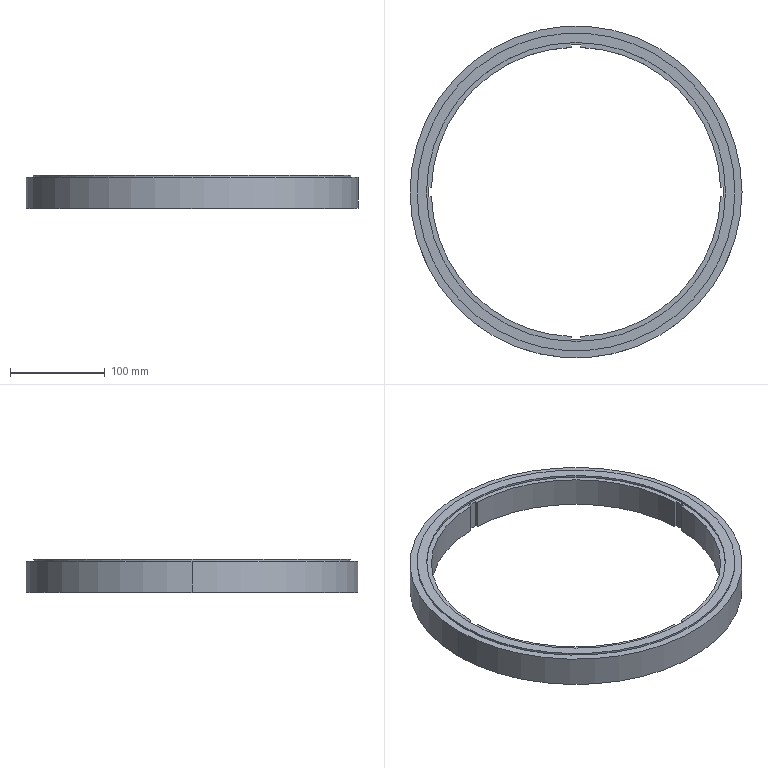Part | SolidWorks | features ICE 6, CirPattern 1, Extrusion 1 | 1 solid | 31 faces | box 350 x 350 x 35 mm | volume 761867 mm3 | plane 17 | cylinder 12 | cone 2 | commonest cylinder face diameters 305 x4 315 x2 330 x2 335 x2 350 x2
STEP:
#1=CARTESIAN_POINT('',(172.,0.,0.));
#2=VERTEX_POINT('',#1);
#3=CARTESIAN_POINT('',(-172.,0.,0.));
#4=VERTEX_POINT('',#3);
#5=CARTESIAN_POINT('',(0.,0.,0.));
#6=DIRECTION('',(0.,0.,-1.));
#7=DIRECTION('',(-1.,0.,0.));
#8=AXIS2_PLACEMENT_3D('',#5,#6,#7);
#9=CIRCLE('',#8,172.);
#10=EDGE_CURVE('',#2,#4,#9,.T.);
#11=ORIENTED_EDGE('',*,*,#10,.F.);
#12=CARTESIAN_POINT('',(175.,0.,0.3684));
#13=VERTEX_POINT('',#12);
#14=CARTESIAN_POINT('',(172.,0.,0.));
#15=DIRECTION('',(0.9925,0.,0.1219));
#16=VECTOR('',#15,1000.);
#17=LINE('',#14,#16);
#18=EDGE_CURVE('',#2,#13,#17,.T.);
#19=ORIENTED_EDGE('',*,*,#18,.T.);
#20=CARTESIAN_POINT('',(-175.,0.,0.3684));
#21=VERTEX_POINT('',#20);
#22=CARTESIAN_POINT('',(0.,0.,0.3684));
#23=DIRECTION('',(0.,0.,-1.));
#24=DIRECTION('',(1.,0.,0.));
#25=AXIS2_PLACEMENT_3D('',#22,#23,#24);
#26=CIRCLE('',#25,175.);
#27=EDGE_CURVE('',#13,#21,#26,.T.);
#28=ORIENTED_EDGE('',*,*,#27,.T.);
#29=CARTESIAN_POINT('',(-172.,0.,0.));
#30=DIRECTION('',(-0.9925,0.,0.1219));
#31=VECTOR('',#30,1000.);
#32=LINE('',#29,#31);
#33=EDGE_CURVE('',#4,#21,#32,.T.);
#34=ORIENTED_EDGE('',*,*,#33,.F.);
#35=EDGE_LOOP('',(#11,#19,#28,#34));
#36=FACE_OUTER_BOUND('',#35,.T.);
#37=CARTESIAN_POINT('',(0.,0.,0.));
#38=DIRECTION('',(0.,0.,1.));
#39=DIRECTION('',(-1.,0.,0.));
#40=AXIS2_PLACEMENT_3D('',#37,#38,#39);
#41=CONICAL_SURFACE('',#40,172.,1.449);
#42=ADVANCED_FACE('',(#36),#41,.T.);
#43=CARTESIAN_POINT('',(165.,0.,1.5));
#44=VERTEX_POINT('',#43);
#45=CARTESIAN_POINT('',(-165.,0.,1.5));
#46=VERTEX_POINT('',#45);
#47=CARTESIAN_POINT('',(0.,0.,1.5));
#48=DIRECTION('',(0.,0.,-1.));
#49=DIRECTION('',(-1.,0.,0.));
#50=AXIS2_PLACEMENT_3D('',#47,#48,#49);
#51=CIRCLE('',#50,165.);
#52=EDGE_CURVE('',#44,#46,#51,.T.);
#53=ORIENTED_EDGE('',*,*,#52,.F.);
#54=CARTESIAN_POINT('',(165.,0.,0.));
#55=VERTEX_POINT('',#54);
#56=CARTESIAN_POINT('',(165.,0.,1.5));
#57=DIRECTION('',(0.,0.,-1.));
#58=VECTOR('',#57,1000.);
#59=LINE('',#56,#58);
#60=EDGE_CURVE('',#44,#55,#59,.T.);
#61=ORIENTED_EDGE('',*,*,#60,.T.);
#62=CARTESIAN_POINT('',(-165.,0.,0.));
#63=VERTEX_POINT('',#62);
#64=CARTESIAN_POINT('',(0.,0.,0.));
#65=DIRECTION('',(0.,0.,-1.));
#66=DIRECTION('',(-1.,0.,0.));
#67=AXIS2_PLACEMENT_3D('',#64,#65,#66);
#68=CIRCLE('',#67,165.);
#69=EDGE_CURVE('',#55,#63,#68,.T.);
#70=ORIENTED_EDGE('',*,*,#69,.T.);
#71=CARTESIAN_POINT('',(-165.,0.,1.5));
#72=DIRECTION('',(0.,0.,-1.));
#73=VECTOR('',#72,1000.);
#74=LINE('',#71,#73);
#75=EDGE_CURVE('',#46,#63,#74,.T.);
#76=ORIENTED_EDGE('',*,*,#75,.F.);
#77=EDGE_LOOP('',(#53,#61,#70,#76));
#78=FACE_OUTER_BOUND('',#77,.T.);
#79=CARTESIAN_POINT('',(0.,0.,1.5));
#80=DIRECTION('',(0.,0.,-1.));
#81=DIRECTION('',(-1.,0.,0.));
#82=AXIS2_PLACEMENT_3D('',#79,#80,#81);
#83=CYLINDRICAL_SURFACE('',#82,165.);
#84=ADVANCED_FACE('',(#78),#83,.F.);
#85=CARTESIAN_POINT('',(-157.5,0.,33.));
#86=VERTEX_POINT('',#85);
#87=CARTESIAN_POINT('',(157.5,0.,33.));
#88=VERTEX_POINT('',#87);
#89=CARTESIAN_POINT('',(0.,0.,33.));
#90=DIRECTION('',(0.,0.,1.));
#91=DIRECTION('',(1.,0.,0.));
#92=AXIS2_PLACEMENT_3D('',#89,#90,#91);
#93=CIRCLE('',#92,157.5);
#94=EDGE_CURVE('',#86,#88,#93,.T.);
#95=ORIENTED_EDGE('',*,*,#94,.F.);
#96=CARTESIAN_POINT('',(-157.5,0.,35.));
#97=VERTEX_POINT('',#96);
#98=CARTESIAN_POINT('',(-157.5,0.,33.));
#99=DIRECTION('',(0.,0.,1.));
#100=VECTOR('',#99,1000.);
#101=LINE('',#98,#100);
#102=EDGE_CURVE('',#86,#97,#101,.T.);
#103=ORIENTED_EDGE('',*,*,#102,.T.);
#104=CARTESIAN_POINT('',(157.5,0.,35.));
#105=VERTEX_POINT('',#104);
#106=CARTESIAN_POINT('',(0.,0.,35.));
#107=DIRECTION('',(0.,0.,1.));
#108=DIRECTION('',(1.,0.,0.));
#109=AXIS2_PLACEMENT_3D('',#106,#107,#108);
#110=CIRCLE('',#109,157.5);
#111=EDGE_CURVE('',#97,#105,#110,.T.);
#112=ORIENTED_EDGE('',*,*,#111,.T.);
#113=CARTESIAN_POINT('',(157.5,0.,33.));
#114=DIRECTION('',(0.,0.,1.));
#115=VECTOR('',#114,1000.);
#116=LINE('',#113,#115);
#117=EDGE_CURVE('',#88,#105,#116,.T.);
#118=ORIENTED_EDGE('',*,*,#117,.F.);
#119=EDGE_LOOP('',(#95,#103,#112,#118));
#120=FACE_OUTER_BOUND('',#119,.T.);
#121=CARTESIAN_POINT('',(0.,0.,33.));
#122=DIRECTION('',(0.,0.,1.));
#123=DIRECTION('',(1.,0.,0.));
#124=AXIS2_PLACEMENT_3D('',#121,#122,#123);
#125=CYLINDRICAL_SURFACE('',#124,157.5);
#126=ADVANCED_FACE('',(#120),#125,.F.);
#127=CARTESIAN_POINT('',(167.5,0.,33.));
#128=VERTEX_POINT('',#127);
#129=CARTESIAN_POINT('',(-167.5,0.,33.));
#130=VERTEX_POINT('',#129);
#131=CARTESIAN_POINT('',(0.,0.,33.));
#132=DIRECTION('',(0.,0.,1.));
#133=DIRECTION('',(1.,0.,0.));
#134=AXIS2_PLACEMENT_3D('',#131,#132,#133);
#135=CIRCLE('',#134,167.5);
#136=EDGE_CURVE('',#128,#130,#135,.T.);
#137=ORIENTED_EDGE('',*,*,#136,.T.);
#138=CARTESIAN_POINT('',(-167.5,0.,35.));
#139=VERTEX_POINT('',#138);
#140=CARTESIAN_POINT('',(-167.5,0.,33.));
#141=DIRECTION('',(0.,0.,1.));
#142=VECTOR('',#141,1000.);
#143=LINE('',#140,#142);
#144=EDGE_CURVE('',#130,#139,#143,.T.);
#145=ORIENTED_EDGE('',*,*,#144,.T.);
#146=CARTESIAN_POINT('',(167.5,0.,35.));
#147=VERTEX_POINT('',#146);
#148=CARTESIAN_POINT('',(0.,0.,35.));
#149=DIRECTION('',(0.,0.,1.));
#150=DIRECTION('',(1.,0.,0.));
#151=AXIS2_PLACEMENT_3D('',#148,#149,#150);
#152=CIRCLE('',#151,167.5);
#153=EDGE_CURVE('',#147,#139,#152,.T.);
#154=ORIENTED_EDGE('',*,*,#153,.F.);
#155=CARTESIAN_POINT('',(167.5,0.,33.));
#156=DIRECTION('',(0.,0.,1.));
#157=VECTOR('',#156,1000.);
#158=LINE('',#155,#157);
#159=EDGE_CURVE('',#128,#147,#158,.T.);
#160=ORIENTED_EDGE('',*,*,#159,.F.);
#161=EDGE_LOOP('',(#137,#145,#154,#160));
#162=FACE_OUTER_BOUND('',#161,.T.);
#163=CARTESIAN_POINT('',(0.,0.,33.));
#164=DIRECTION('',(0.,0.,1.));
#165=DIRECTION('',(1.,0.,0.));
#166=AXIS2_PLACEMENT_3D('',#163,#164,#165);
#167=CYLINDRICAL_SURFACE('',#166,167.5);
#168=ADVANCED_FACE('',(#162),#167,.T.);
#169=CARTESIAN_POINT('',(175.,0.,33.));
#170=VERTEX_POINT('',#169);
#171=CARTESIAN_POINT('',(-175.,0.,33.));
#172=VERTEX_POINT('',#171);
#173=CARTESIAN_POINT('',(0.,0.,33.));
#174=DIRECTION('',(0.,0.,1.));
#175=DIRECTION('',(1.,0.,0.));
#176=AXIS2_PLACEMENT_3D('',#173,#174,#175);
#177=CIRCLE('',#176,175.);
#178=EDGE_CURVE('',#170,#172,#177,.T.);
#179=ORIENTED_EDGE('',*,*,#178,.F.);
#180=CARTESIAN_POINT('',(175.,0.,35.));
#181=DIRECTION('',(0.,0.,-1.));
#182=VECTOR('',#181,1000.);
#183=LINE('',#180,#182);
#184=EDGE_CURVE('',#170,#13,#183,.T.);
#185=ORIENTED_EDGE('',*,*,#184,.T.);
#186=CARTESIAN_POINT('',(0.,0.,0.3684));
#187=DIRECTION('',(0.,0.,-1.));
#188=DIRECTION('',(1.,0.,0.));
#189=AXIS2_PLACEMENT_3D('',#186,#187,#188);
#190=CIRCLE('',#189,175.);
#191=EDGE_CURVE('',#21,#13,#190,.T.);
#192=ORIENTED_EDGE('',*,*,#191,.F.);
#193=CARTESIAN_POINT('',(-175.,0.,35.));
#194=DIRECTION('',(0.,0.,-1.));
#195=VECTOR('',#194,1000.);
#196=LINE('',#193,#195);
#197=EDGE_CURVE('',#172,#21,#196,.T.);
#198=ORIENTED_EDGE('',*,*,#197,.F.);
#199=EDGE_LOOP('',(#179,#185,#192,#198));
#200=FACE_OUTER_BOUND('',#199,.T.);
#201=CARTESIAN_POINT('',(0.,0.,35.));
#202=DIRECTION('',(0.,0.,-1.));
#203=DIRECTION('',(-1.,0.,0.));
#204=AXIS2_PLACEMENT_3D('',#201,#202,#203);
#205=CYLINDRICAL_SURFACE('',#204,175.);
#206=ADVANCED_FACE('',(#200),#205,.T.);
#207=ORIENTED_EDGE('',*,*,#184,.F.);
#208=CARTESIAN_POINT('',(0.,0.,33.));
#209=DIRECTION('',(0.,0.,1.));
#210=DIRECTION('',(1.,0.,0.));
#211=AXIS2_PLACEMENT_3D('',#208,#209,#210);
#212=CIRCLE('',#211,175.);
#213=EDGE_CURVE('',#172,#170,#212,.T.);
#214=ORIENTED_EDGE('',*,*,#213,.F.);
#215=ORIENTED_EDGE('',*,*,#197,.T.);
#216=ORIENTED_EDGE('',*,*,#27,.F.);
#217=EDGE_LOOP('',(#207,#214,#215,#216));
#218=FACE_OUTER_BOUND('',#217,.T.);
#219=CARTESIAN_POINT('',(0.,0.,35.));
#220=DIRECTION('',(0.,0.,-1.));
#221=DIRECTION('',(-1.,0.,0.));
#222=AXIS2_PLACEMENT_3D('',#219,#220,#221);
#223=CYLINDRICAL_SURFACE('',#222,175.);
#224=ADVANCED_FACE('',(#218),#223,.T.);
#225=CARTESIAN_POINT('',(0.,0.,0.));
#226=DIRECTION('',(0.,0.,-1.));
#227=DIRECTION('',(-1.,0.,0.));
#228=AXIS2_PLACEMENT_3D('',#225,#226,#227);
#229=CIRCLE('',#228,165.);
#230=EDGE_CURVE('',#63,#55,#229,.T.);
#231=ORIENTED_EDGE('',*,*,#230,.F.);
#232=ORIENTED_EDGE('',*,*,#69,.F.);
#233=EDGE_LOOP('',(#231,#232));
#234=FACE_BOUND('',#233,.T.);
#235=CARTESIAN_POINT('',(0.,0.,0.));
#236=DIRECTION('',(0.,0.,-1.));
#237=DIRECTION('',(-1.,0.,0.));
#238=AXIS2_PLACEMENT_3D('',#235,#236,#237);
#239=CIRCLE('',#238,172.);
#240=EDGE_CURVE('',#4,#2,#239,.T.);
#241=ORIENTED_EDGE('',*,*,#240,.T.);
#242=ORIENTED_EDGE('',*,*,#10,.T.);
#243=EDGE_LOOP('',(#241,#242));
#244=FACE_OUTER_BOUND('',#243,.T.);
#245=CARTESIAN_POINT('',(0.,0.,0.));
#246=DIRECTION('',(0.,0.,1.));
#247=DIRECTION('',(1.,0.,0.));
#248=AXIS2_PLACEMENT_3D('',#245,#246,#247);
#249=PLANE('',#248);
#250=ADVANCED_FACE('',(#234,#244),#249,.F.);
#251=CARTESIAN_POINT('',(-5.,-152.418,1.5));
#252=VERTEX_POINT('',#251);
#253=CARTESIAN_POINT('',(-152.418,-5.,1.5));
#254=VERTEX_POINT('',#253);
#255=CARTESIAN_POINT('',(0.,0.,1.5));
#256=DIRECTION('',(0.,0.,-1.));
#257=DIRECTION('',(-1.,0.,0.));
#258=AXIS2_PLACEMENT_3D('',#255,#256,#257);
#259=CIRCLE('',#258,152.5);
#260=EDGE_CURVE('',#252,#254,#259,.T.);
#261=ORIENTED_EDGE('',*,*,#260,.T.);
#262=CARTESIAN_POINT('',(-152.418,-5.,33.));
#263=VERTEX_POINT('',#262);
#264=CARTESIAN_POINT('',(-152.418,-5.,35.));
#265=DIRECTION('',(0.,0.,1.));
#266=VECTOR('',#265,1000.);
#267=LINE('',#264,#266);
#268=EDGE_CURVE('',#254,#263,#267,.T.);
#269=ORIENTED_EDGE('',*,*,#268,.T.);
#270=CARTESIAN_POINT('',(-5.,-152.418,33.));
#271=VERTEX_POINT('',#270);
#272=CARTESIAN_POINT('',(0.,0.,33.));
#273=DIRECTION('',(0.,0.,1.));
#274=DIRECTION('',(1.,0.,0.));
#275=AXIS2_PLACEMENT_3D('',#272,#273,#274);
#276=CIRCLE('',#275,152.5);
#277=EDGE_CURVE('',#263,#271,#276,.T.);
#278=ORIENTED_EDGE('',*,*,#277,.T.);
#279=CARTESIAN_POINT('',(-5.,-152.418,35.));
#280=DIRECTION('',(0.,0.,-1.));
#281=VECTOR('',#280,1000.);
#282=LINE('',#279,#281);
#283=EDGE_CURVE('',#271,#252,#282,.T.);
#284=ORIENTED_EDGE('',*,*,#283,.T.);
#285=EDGE_LOOP('',(#261,#269,#278,#284));
#286=FACE_OUTER_BOUND('',#285,.T.);
#287=CARTESIAN_POINT('',(0.,0.,35.));
#288=DIRECTION('',(0.,0.,-1.));
#289=DIRECTION('',(-1.,0.,0.));
#290=AXIS2_PLACEMENT_3D('',#287,#288,#289);
#291=CYLINDRICAL_SURFACE('',#290,152.5);
#292=ADVANCED_FACE('',(#286),#291,.F.);
#293=CARTESIAN_POINT('',(5.,-152.418,33.));
#294=VERTEX_POINT('',#293);
#295=CARTESIAN_POINT('',(152.418,-5.,33.));
#296=VERTEX_POINT('',#295);
#297=CARTESIAN_POINT('',(0.,0.,33.));
#298=DIRECTION('',(0.,0.,1.));
#299=DIRECTION('',(1.,0.,0.));
#300=AXIS2_PLACEMENT_3D('',#297,#298,#299);
#301=CIRCLE('',#300,152.5);
#302=EDGE_CURVE('',#294,#296,#301,.T.);
#303=ORIENTED_EDGE('',*,*,#302,.T.);
#304=CARTESIAN_POINT('',(152.418,-5.,1.5));
#305=VERTEX_POINT('',#304);
#306=CARTESIAN_POINT('',(152.418,-5.,35.));
#307=DIRECTION('',(0.,0.,-1.));
#308=VECTOR('',#307,1000.);
#309=LINE('',#306,#308);
#310=EDGE_CURVE('',#296,#305,#309,.T.);
#311=ORIENTED_EDGE('',*,*,#310,.T.);
#312=CARTESIAN_POINT('',(5.,-152.418,1.5));
#313=VERTEX_POINT('',#312);
#314=CARTESIAN_POINT('',(0.,0.,1.5));
#315=DIRECTION('',(0.,0.,-1.));
#316=DIRECTION('',(-1.,0.,0.));
#317=AXIS2_PLACEMENT_3D('',#314,#315,#316);
#318=CIRCLE('',#317,152.5);
#319=EDGE_CURVE('',#305,#313,#318,.T.);
#320=ORIENTED_EDGE('',*,*,#319,.T.);
#321=CARTESIAN_POINT('',(5.,-152.418,35.));
#322=DIRECTION('',(0.,0.,1.));
#323=VECTOR('',#322,1000.);
#324=LINE('',#321,#323);
#325=EDGE_CURVE('',#313,#294,#324,.T.);
#326=ORIENTED_EDGE('',*,*,#325,.T.);
#327=EDGE_LOOP('',(#303,#311,#320,#326));
#328=FACE_OUTER_BOUND('',#327,.T.);
#329=CARTESIAN_POINT('',(0.,0.,35.));
#330=DIRECTION('',(0.,0.,-1.));
#331=DIRECTION('',(-1.,0.,0.));
#332=AXIS2_PLACEMENT_3D('',#329,#330,#331);
#333=CYLINDRICAL_SURFACE('',#332,152.5);
#334=ADVANCED_FACE('',(#328),#333,.F.);
#335=CARTESIAN_POINT('',(-5.,152.418,33.));
#336=VERTEX_POINT('',#335);
#337=CARTESIAN_POINT('',(-152.418,5.,33.));
#338=VERTEX_POINT('',#337);
#339=CARTESIAN_POINT('',(0.,0.,33.));
#340=DIRECTION('',(0.,0.,1.));
#341=DIRECTION('',(1.,0.,0.));
#342=AXIS2_PLACEMENT_3D('',#339,#340,#341);
#343=CIRCLE('',#342,152.5);
#344=EDGE_CURVE('',#336,#338,#343,.T.);
#345=ORIENTED_EDGE('',*,*,#344,.T.);
#346=CARTESIAN_POINT('',(-152.418,5.,1.5));
#347=VERTEX_POINT('',#346);
#348=CARTESIAN_POINT('',(-152.418,5.,35.));
#349=DIRECTION('',(0.,0.,-1.));
#350=VECTOR('',#349,1000.);
#351=LINE('',#348,#350);
#352=EDGE_CURVE('',#338,#347,#351,.T.);
#353=ORIENTED_EDGE('',*,*,#352,.T.);
#354=CARTESIAN_POINT('',(-5.,152.418,1.5));
#355=VERTEX_POINT('',#354);
#356=CARTESIAN_POINT('',(0.,0.,1.5));
#357=DIRECTION('',(0.,0.,-1.));
#358=DIRECTION('',(-1.,0.,0.));
#359=AXIS2_PLACEMENT_3D('',#356,#357,#358);
#360=CIRCLE('',#359,152.5);
#361=EDGE_CURVE('',#347,#355,#360,.T.);
#362=ORIENTED_EDGE('',*,*,#361,.T.);
#363=CARTESIAN_POINT('',(-5.,152.418,35.));
#364=DIRECTION('',(0.,0.,1.));
#365=VECTOR('',#364,1000.);
#366=LINE('',#363,#365);
#367=EDGE_CURVE('',#355,#336,#366,.T.);
#368=ORIENTED_EDGE('',*,*,#367,.T.);
#369=EDGE_LOOP('',(#345,#353,#362,#368));
#370=FACE_OUTER_BOUND('',#369,.T.);
#371=CARTESIAN_POINT('',(0.,0.,35.));
#372=DIRECTION('',(0.,0.,-1.));
#373=DIRECTION('',(-1.,0.,0.));
#374=AXIS2_PLACEMENT_3D('',#371,#372,#373);
#375=CYLINDRICAL_SURFACE('',#374,152.5);
#376=ADVANCED_FACE('',(#370),#375,.F.);
#377=ORIENTED_EDGE('',*,*,#136,.F.);
#378=CARTESIAN_POINT('',(0.,0.,33.));
#379=DIRECTION('',(0.,0.,1.));
#380=DIRECTION('',(1.,0.,0.));
#381=AXIS2_PLACEMENT_3D('',#378,#379,#380);
#382=CIRCLE('',#381,167.5);
#383=EDGE_CURVE('',#130,#128,#382,.T.);
#384=ORIENTED_EDGE('',*,*,#383,.F.);
#385=EDGE_LOOP('',(#377,#384));
#386=FACE_BOUND('',#385,.T.);
#387=ORIENTED_EDGE('',*,*,#213,.T.);
#388=ORIENTED_EDGE('',*,*,#178,.T.);
#389=EDGE_LOOP('',(#387,#388));
#390=FACE_OUTER_BOUND('',#389,.T.);
#391=CARTESIAN_POINT('',(0.,0.,33.));
#392=DIRECTION('',(0.,0.,1.));
#393=DIRECTION('',(1.,0.,0.));
#394=AXIS2_PLACEMENT_3D('',#391,#392,#393);
#395=PLANE('',#394);
#396=ADVANCED_FACE('',(#386,#390),#395,.T.);
#397=ORIENTED_EDGE('',*,*,#144,.F.);
#398=ORIENTED_EDGE('',*,*,#383,.T.);
#399=ORIENTED_EDGE('',*,*,#159,.T.);
#400=CARTESIAN_POINT('',(0.,0.,35.));
#401=DIRECTION('',(0.,0.,1.));
#402=DIRECTION('',(1.,0.,0.));
#403=AXIS2_PLACEMENT_3D('',#400,#401,#402);
#404=CIRCLE('',#403,167.5);
#405=EDGE_CURVE('',#139,#147,#404,.T.);
#406=ORIENTED_EDGE('',*,*,#405,.F.);
#407=EDGE_LOOP('',(#397,#398,#399,#406));
#408=FACE_OUTER_BOUND('',#407,.T.);
#409=CARTESIAN_POINT('',(0.,0.,33.));
#410=DIRECTION('',(0.,0.,1.));
#411=DIRECTION('',(1.,0.,0.));
#412=AXIS2_PLACEMENT_3D('',#409,#410,#411);
#413=CYLINDRICAL_SURFACE('',#412,167.5);
#414=ADVANCED_FACE('',(#408),#413,.T.);
#415=CARTESIAN_POINT('',(0.,0.,35.));
#416=DIRECTION('',(0.,0.,1.));
#417=DIRECTION('',(1.,0.,0.));
#418=AXIS2_PLACEMENT_3D('',#415,#416,#417);
#419=CIRCLE('',#418,157.5);
#420=EDGE_CURVE('',#105,#97,#419,.T.);
#421=ORIENTED_EDGE('',*,*,#420,.F.);
#422=ORIENTED_EDGE('',*,*,#111,.F.);
#423=EDGE_LOOP('',(#421,#422));
#424=FACE_BOUND('',#423,.T.);
#425=ORIENTED_EDGE('',*,*,#153,.T.);
#426=ORIENTED_EDGE('',*,*,#405,.T.);
#427=EDGE_LOOP('',(#425,#426));
#428=FACE_OUTER_BOUND('',#427,.T.);
#429=CARTESIAN_POINT('',(0.,0.,35.));
#430=DIRECTION('',(0.,0.,1.));
#431=DIRECTION('',(1.,0.,0.));
#432=AXIS2_PLACEMENT_3D('',#429,#430,#431);
#433=PLANE('',#432);
#434=ADVANCED_FACE('',(#424,#428),#433,.T.);
#435=ORIENTED_EDGE('',*,*,#102,.F.);
#436=CARTESIAN_POINT('',(0.,0.,33.));
#437=DIRECTION('',(0.,0.,1.));
#438=DIRECTION('',(1.,0.,0.));
#439=AXIS2_PLACEMENT_3D('',#436,#437,#438);
#440=CIRCLE('',#439,157.5);
#441=EDGE_CURVE('',#88,#86,#440,.T.);
#442=ORIENTED_EDGE('',*,*,#441,.F.);
#443=ORIENTED_EDGE('',*,*,#117,.T.);
#444=ORIENTED_EDGE('',*,*,#420,.T.);
#445=EDGE_LOOP('',(#435,#442,#443,#444));
#446=FACE_OUTER_BOUND('',#445,.T.);
#447=CARTESIAN_POINT('',(0.,0.,33.));
#448=DIRECTION('',(0.,0.,1.));
#449=DIRECTION('',(1.,0.,0.));
#450=AXIS2_PLACEMENT_3D('',#447,#448,#449);
#451=CYLINDRICAL_SURFACE('',#450,157.5);
#452=ADVANCED_FACE('',(#446),#451,.F.);
#453=CARTESIAN_POINT('',(155.,-5.,33.));
#454=VERTEX_POINT('',#453);
#455=CARTESIAN_POINT('',(0.,-5.,33.));
#456=DIRECTION('',(1.,0.,0.));
#457=VECTOR('',#456,1000.);
#458=LINE('',#455,#457);
#459=EDGE_CURVE('',#296,#454,#458,.T.);
#460=ORIENTED_EDGE('',*,*,#459,.F.);
#461=ORIENTED_EDGE('',*,*,#302,.F.);
#462=CARTESIAN_POINT('',(5.,-155.,33.));
#463=VERTEX_POINT('',#462);
#464=CARTESIAN_POINT('',(5.,0.,33.));
#465=DIRECTION('',(0.,1.,0.));
#466=VECTOR('',#465,1000.);
#467=LINE('',#464,#466);
#468=EDGE_CURVE('',#463,#294,#467,.T.);
#469=ORIENTED_EDGE('',*,*,#468,.F.);
#470=CARTESIAN_POINT('',(-5.,-155.,33.));
#471=VERTEX_POINT('',#470);
#472=CARTESIAN_POINT('',(0.,-155.,33.));
#473=DIRECTION('',(1.,0.,0.));
#474=VECTOR('',#473,1000.);
#475=LINE('',#472,#474);
#476=EDGE_CURVE('',#471,#463,#475,.T.);
#477=ORIENTED_EDGE('',*,*,#476,.F.);
#478=CARTESIAN_POINT('',(-5.,0.,33.));
#479=DIRECTION('',(0.,-1.,0.));
#480=VECTOR('',#479,1000.);
#481=LINE('',#478,#480);
#482=EDGE_CURVE('',#271,#471,#481,.T.);
#483=ORIENTED_EDGE('',*,*,#482,.F.);
#484=ORIENTED_EDGE('',*,*,#277,.F.);
#485=CARTESIAN_POINT('',(-155.,-5.,33.));
#486=VERTEX_POINT('',#485);
#487=CARTESIAN_POINT('',(0.,-5.,33.));
#488=DIRECTION('',(1.,0.,0.));
#489=VECTOR('',#488,1000.);
#490=LINE('',#487,#489);
#491=EDGE_CURVE('',#486,#263,#490,.T.);
#492=ORIENTED_EDGE('',*,*,#491,.F.);
#493=CARTESIAN_POINT('',(-155.,5.,33.));
#494=VERTEX_POINT('',#493);
#495=CARTESIAN_POINT('',(-155.,0.,33.));
#496=DIRECTION('',(0.,-1.,0.));
#497=VECTOR('',#496,1000.);
#498=LINE('',#495,#497);
#499=EDGE_CURVE('',#494,#486,#498,.T.);
#500=ORIENTED_EDGE('',*,*,#499,.F.);
#501=CARTESIAN_POINT('',(0.,5.,33.));
#502=DIRECTION('',(-1.,0.,0.));
#503=VECTOR('',#502,1000.);
#504=LINE('',#501,#503);
#505=EDGE_CURVE('',#338,#494,#504,.T.);
#506=ORIENTED_EDGE('',*,*,#505,.F.);
#507=ORIENTED_EDGE('',*,*,#344,.F.);
#508=CARTESIAN_POINT('',(-5.,155.,33.));
#509=VERTEX_POINT('',#508);
#510=CARTESIAN_POINT('',(-5.,0.,33.));
#511=DIRECTION('',(0.,-1.,0.));
#512=VECTOR('',#511,1000.);
#513=LINE('',#510,#512);
#514=EDGE_CURVE('',#509,#336,#513,.T.);
#515=ORIENTED_EDGE('',*,*,#514,.F.);
#516=CARTESIAN_POINT('',(5.,155.,33.));
#517=VERTEX_POINT('',#516);
#518=CARTESIAN_POINT('',(0.,155.,33.));
#519=DIRECTION('',(-1.,0.,0.));
#520=VECTOR('',#519,1000.);
#521=LINE('',#518,#520);
#522=EDGE_CURVE('',#517,#509,#521,.T.);
#523=ORIENTED_EDGE('',*,*,#522,.F.);
#524=CARTESIAN_POINT('',(5.,152.418,33.));
#525=VERTEX_POINT('',#524);
#526=CARTESIAN_POINT('',(5.,0.,33.));
#527=DIRECTION('',(0.,1.,0.));
#528=VECTOR('',#527,1000.);
#529=LINE('',#526,#528);
#530=EDGE_CURVE('',#525,#517,#529,.T.);
#531=ORIENTED_EDGE('',*,*,#530,.F.);
#532=CARTESIAN_POINT('',(152.418,5.,33.));
#533=VERTEX_POINT('',#532);
#534=CARTESIAN_POINT('',(0.,0.,33.));
#535=DIRECTION('',(0.,0.,1.));
#536=DIRECTION('',(1.,0.,0.));
#537=AXIS2_PLACEMENT_3D('',#534,#535,#536);
#538=CIRCLE('',#537,152.5);
#539=EDGE_CURVE('',#533,#525,#538,.T.);
#540=ORIENTED_EDGE('',*,*,#539,.F.);
#541=CARTESIAN_POINT('',(155.,5.,33.));
#542=VERTEX_POINT('',#541);
#543=CARTESIAN_POINT('',(0.,5.,33.));
#544=DIRECTION('',(-1.,0.,0.));
#545=VECTOR('',#544,1000.);
#546=LINE('',#543,#545);
#547=EDGE_CURVE('',#542,#533,#546,.T.);
#548=ORIENTED_EDGE('',*,*,#547,.F.);
#549=CARTESIAN_POINT('',(155.,0.,33.));
#550=DIRECTION('',(0.,1.,0.));
#551=VECTOR('',#550,1000.);
#552=LINE('',#549,#551);
#553=EDGE_CURVE('',#454,#542,#552,.T.);
#554=ORIENTED_EDGE('',*,*,#553,.F.);
#555=EDGE_LOOP('',(#460,#461,#469,#477,#483,#484,#492,#500,#506,#507,#515,#523,#531,#540,#548,#554));
#556=FACE_BOUND('',#555,.T.);
#557=ORIENTED_EDGE('',*,*,#441,.T.);
#558=ORIENTED_EDGE('',*,*,#94,.T.);
#559=EDGE_LOOP('',(#557,#558));
#560=FACE_OUTER_BOUND('',#559,.T.);
#561=CARTESIAN_POINT('',(0.,0.,33.));
#562=DIRECTION('',(0.,0.,1.));
#563=DIRECTION('',(1.,0.,0.));
#564=AXIS2_PLACEMENT_3D('',#561,#562,#563);
#565=PLANE('',#564);
#566=ADVANCED_FACE('',(#556,#560),#565,.T.);
#567=ORIENTED_EDGE('',*,*,#60,.F.);
#568=CARTESIAN_POINT('',(0.,0.,1.5));
#569=DIRECTION('',(0.,0.,-1.));
#570=DIRECTION('',(-1.,0.,0.));
#571=AXIS2_PLACEMENT_3D('',#568,#569,#570);
#572=CIRCLE('',#571,165.);
#573=EDGE_CURVE('',#46,#44,#572,.T.);
#574=ORIENTED_EDGE('',*,*,#573,.F.);
#575=ORIENTED_EDGE('',*,*,#75,.T.);
#576=ORIENTED_EDGE('',*,*,#230,.T.);
#577=EDGE_LOOP('',(#567,#574,#575,#576));
#578=FACE_OUTER_BOUND('',#577,.T.);
#579=CARTESIAN_POINT('',(0.,0.,1.5));
#580=DIRECTION('',(0.,0.,-1.));
#581=DIRECTION('',(-1.,0.,0.));
#582=AXIS2_PLACEMENT_3D('',#579,#580,#581);
#583=CYLINDRICAL_SURFACE('',#582,165.);
#584=ADVANCED_FACE('',(#578),#583,.F.);
#585=CARTESIAN_POINT('',(155.,-5.,1.5));
#586=VERTEX_POINT('',#585);
#587=CARTESIAN_POINT('',(155.,-5.,1.5));
#588=DIRECTION('',(-1.,0.,0.));
#589=VECTOR('',#588,1000.);
#590=LINE('',#587,#589);
#591=EDGE_CURVE('',#586,#305,#590,.T.);
#592=ORIENTED_EDGE('',*,*,#591,.F.);
#593=CARTESIAN_POINT('',(155.,5.,1.5));
#594=VERTEX_POINT('',#593);
#595=CARTESIAN_POINT('',(155.,5.,1.5));
#596=DIRECTION('',(0.,-1.,0.));
#597=VECTOR('',#596,1000.);
#598=LINE('',#595,#597);
#599=EDGE_CURVE('',#594,#586,#598,.T.);
#600=ORIENTED_EDGE('',*,*,#599,.F.);
#601=CARTESIAN_POINT('',(152.418,5.,1.5));
#602=VERTEX_POINT('',#601);
#603=CARTESIAN_POINT('',(155.,5.,1.5));
#604=DIRECTION('',(1.,0.,0.));
#605=VECTOR('',#604,1000.);
#606=LINE('',#603,#605);
#607=EDGE_CURVE('',#602,#594,#606,.T.);
#608=ORIENTED_EDGE('',*,*,#607,.F.);
#609=CARTESIAN_POINT('',(5.,152.418,1.5));
#610=VERTEX_POINT('',#609);
#611=CARTESIAN_POINT('',(0.,0.,1.5));
#612=DIRECTION('',(0.,0.,-1.));
#613=DIRECTION('',(-1.,0.,0.));
#614=AXIS2_PLACEMENT_3D('',#611,#612,#613);
#615=CIRCLE('',#614,152.5);
#616=EDGE_CURVE('',#610,#602,#615,.T.);
#617=ORIENTED_EDGE('',*,*,#616,.F.);
#618=CARTESIAN_POINT('',(5.,155.,1.5));
#619=VERTEX_POINT('',#618);
#620=CARTESIAN_POINT('',(5.,-155.,1.5));
#621=DIRECTION('',(0.,-1.,0.));
#622=VECTOR('',#621,1000.);
#623=LINE('',#620,#622);
#624=EDGE_CURVE('',#619,#610,#623,.T.);
#625=ORIENTED_EDGE('',*,*,#624,.F.);
#626=CARTESIAN_POINT('',(-5.,155.,1.5));
#627=VERTEX_POINT('',#626);
#628=CARTESIAN_POINT('',(5.,155.,1.5));
#629=DIRECTION('',(1.,0.,0.));
#630=VECTOR('',#629,1000.);
#631=LINE('',#628,#630);
#632=EDGE_CURVE('',#627,#619,#631,.T.);
#633=ORIENTED_EDGE('',*,*,#632,.F.);
#634=CARTESIAN_POINT('',(-5.,-155.,1.5));
#635=DIRECTION('',(0.,1.,0.));
#636=VECTOR('',#635,1000.);
#637=LINE('',#634,#636);
#638=EDGE_CURVE('',#355,#627,#637,.T.);
#639=ORIENTED_EDGE('',*,*,#638,.F.);
#640=ORIENTED_EDGE('',*,*,#361,.F.);
#641=CARTESIAN_POINT('',(-155.,5.,1.5));
#642=VERTEX_POINT('',#641);
#643=CARTESIAN_POINT('',(155.,5.,1.5));
#644=DIRECTION('',(1.,0.,0.));
#645=VECTOR('',#644,1000.);
#646=LINE('',#643,#645);
#647=EDGE_CURVE('',#642,#347,#646,.T.);
#648=ORIENTED_EDGE('',*,*,#647,.F.);
#649=CARTESIAN_POINT('',(-155.,-5.,1.5));
#650=VERTEX_POINT('',#649);
#651=CARTESIAN_POINT('',(-155.,5.,1.5));
#652=DIRECTION('',(0.,1.,0.));
#653=VECTOR('',#652,1000.);
#654=LINE('',#651,#653);
#655=EDGE_CURVE('',#650,#642,#654,.T.);
#656=ORIENTED_EDGE('',*,*,#655,.F.);
#657=CARTESIAN_POINT('',(155.,-5.,1.5));
#658=DIRECTION('',(-1.,0.,0.));
#659=VECTOR('',#658,1000.);
#660=LINE('',#657,#659);
#661=EDGE_CURVE('',#254,#650,#660,.T.);
#662=ORIENTED_EDGE('',*,*,#661,.F.);
#663=ORIENTED_EDGE('',*,*,#260,.F.);
#664=CARTESIAN_POINT('',(-5.,-155.,1.5));
#665=VERTEX_POINT('',#664);
#666=CARTESIAN_POINT('',(-5.,-155.,1.5));
#667=DIRECTION('',(0.,1.,0.));
#668=VECTOR('',#667,1000.);
#669=LINE('',#666,#668);
#670=EDGE_CURVE('',#665,#252,#669,.T.);
#671=ORIENTED_EDGE('',*,*,#670,.F.);
#672=CARTESIAN_POINT('',(5.,-155.,1.5));
#673=VERTEX_POINT('',#672);
#674=CARTESIAN_POINT('',(5.,-155.,1.5));
#675=DIRECTION('',(-1.,0.,0.));
#676=VECTOR('',#675,1000.);
#677=LINE('',#674,#676);
#678=EDGE_CURVE('',#673,#665,#677,.T.);
#679=ORIENTED_EDGE('',*,*,#678,.F.);
#680=CARTESIAN_POINT('',(5.,-155.,1.5));
#681=DIRECTION('',(0.,-1.,0.));
#682=VECTOR('',#681,1000.);
#683=LINE('',#680,#682);
#684=EDGE_CURVE('',#313,#673,#683,.T.);
#685=ORIENTED_EDGE('',*,*,#684,.F.);
#686=ORIENTED_EDGE('',*,*,#319,.F.);
#687=EDGE_LOOP('',(#592,#600,#608,#617,#625,#633,#639,#640,#648,#656,#662,#663,#671,#679,#685,#686));
#688=FACE_BOUND('',#687,.T.);
#689=ORIENTED_EDGE('',*,*,#573,.T.);
#690=ORIENTED_EDGE('',*,*,#52,.T.);
#691=EDGE_LOOP('',(#689,#690));
#692=FACE_OUTER_BOUND('',#691,.T.);
#693=CARTESIAN_POINT('',(0.,0.,1.5));
#694=DIRECTION('',(0.,0.,-1.));
#695=DIRECTION('',(-1.,0.,0.));
#696=AXIS2_PLACEMENT_3D('',#693,#694,#695);
#697=PLANE('',#696);
#698=ADVANCED_FACE('',(#688,#692),#697,.T.);
#699=ORIENTED_EDGE('',*,*,#616,.T.);
#700=CARTESIAN_POINT('',(152.418,5.,35.));
#701=DIRECTION('',(0.,0.,1.));
#702=VECTOR('',#701,1000.);
#703=LINE('',#700,#702);
#704=EDGE_CURVE('',#602,#533,#703,.T.);
#705=ORIENTED_EDGE('',*,*,#704,.T.);
#706=ORIENTED_EDGE('',*,*,#539,.T.);
#707=CARTESIAN_POINT('',(5.,152.418,35.));
#708=DIRECTION('',(0.,0.,-1.));
#709=VECTOR('',#708,1000.);
#710=LINE('',#707,#709);
#711=EDGE_CURVE('',#525,#610,#710,.T.);
#712=ORIENTED_EDGE('',*,*,#711,.T.);
#713=EDGE_LOOP('',(#699,#705,#706,#712));
#714=FACE_OUTER_BOUND('',#713,.T.);
#715=CARTESIAN_POINT('',(0.,0.,35.));
#716=DIRECTION('',(0.,0.,-1.));
#717=DIRECTION('',(-1.,0.,0.));
#718=AXIS2_PLACEMENT_3D('',#715,#716,#717);
#719=CYLINDRICAL_SURFACE('',#718,152.5);
#720=ADVANCED_FACE('',(#714),#719,.F.);
#721=ORIENTED_EDGE('',*,*,#514,.T.);
#722=ORIENTED_EDGE('',*,*,#367,.F.);
#723=ORIENTED_EDGE('',*,*,#638,.T.);
#724=CARTESIAN_POINT('',(-5.,155.,101.));
#725=DIRECTION('',(0.,0.,-1.));
#726=VECTOR('',#725,1000.);
#727=LINE('',#724,#726);
#728=EDGE_CURVE('',#509,#627,#727,.T.);
#729=ORIENTED_EDGE('',*,*,#728,.F.);
#730=EDGE_LOOP('',(#721,#722,#723,#729));
#731=FACE_OUTER_BOUND('',#730,.T.);
#732=CARTESIAN_POINT('',(-5.,-155.,101.));
#733=DIRECTION('',(-1.,0.,0.));
#734=DIRECTION('',(0.,-1.,0.));
#735=AXIS2_PLACEMENT_3D('',#732,#733,#734);
#736=PLANE('',#735);
#737=ADVANCED_FACE('',(#731),#736,.F.);
#738=ORIENTED_EDGE('',*,*,#530,.T.);
#739=CARTESIAN_POINT('',(5.,155.,101.));
#740=DIRECTION('',(0.,0.,-1.));
#741=VECTOR('',#740,1000.);
#742=LINE('',#739,#741);
#743=EDGE_CURVE('',#517,#619,#742,.T.);
#744=ORIENTED_EDGE('',*,*,#743,.T.);
#745=ORIENTED_EDGE('',*,*,#624,.T.);
#746=ORIENTED_EDGE('',*,*,#711,.F.);
#747=EDGE_LOOP('',(#738,#744,#745,#746));
#748=FACE_OUTER_BOUND('',#747,.T.);
#749=CARTESIAN_POINT('',(5.,-155.,101.));
#750=DIRECTION('',(1.,0.,0.));
#751=DIRECTION('',(0.,0.,-1.));
#752=AXIS2_PLACEMENT_3D('',#749,#750,#751);
#753=PLANE('',#752);
#754=ADVANCED_FACE('',(#748),#753,.F.);
#755=ORIENTED_EDGE('',*,*,#522,.T.);
#756=ORIENTED_EDGE('',*,*,#728,.T.);
#757=ORIENTED_EDGE('',*,*,#632,.T.);
#758=ORIENTED_EDGE('',*,*,#743,.F.);
#759=EDGE_LOOP('',(#755,#756,#757,#758));
#760=FACE_OUTER_BOUND('',#759,.T.);
#761=CARTESIAN_POINT('',(5.,155.,101.));
#762=DIRECTION('',(0.,1.,0.));
#763=DIRECTION('',(-1.,0.,0.));
#764=AXIS2_PLACEMENT_3D('',#761,#762,#763);
#765=PLANE('',#764);
#766=ADVANCED_FACE('',(#760),#765,.F.);
#767=ORIENTED_EDGE('',*,*,#468,.T.);
#768=ORIENTED_EDGE('',*,*,#325,.F.);
#769=ORIENTED_EDGE('',*,*,#684,.T.);
#770=CARTESIAN_POINT('',(5.,-155.,101.));
#771=DIRECTION('',(0.,0.,-1.));
#772=VECTOR('',#771,1000.);
#773=LINE('',#770,#772);
#774=EDGE_CURVE('',#463,#673,#773,.T.);
#775=ORIENTED_EDGE('',*,*,#774,.F.);
#776=EDGE_LOOP('',(#767,#768,#769,#775));
#777=FACE_OUTER_BOUND('',#776,.T.);
#778=CARTESIAN_POINT('',(5.,-155.,101.));
#779=DIRECTION('',(1.,0.,0.));
#780=DIRECTION('',(0.,0.,-1.));
#781=AXIS2_PLACEMENT_3D('',#778,#779,#780);
#782=PLANE('',#781);
#783=ADVANCED_FACE('',(#777),#782,.F.);
#784=ORIENTED_EDGE('',*,*,#482,.T.);
#785=CARTESIAN_POINT('',(-5.,-155.,101.));
#786=DIRECTION('',(0.,0.,-1.));
#787=VECTOR('',#786,1000.);
#788=LINE('',#785,#787);
#789=EDGE_CURVE('',#471,#665,#788,.T.);
#790=ORIENTED_EDGE('',*,*,#789,.T.);
#791=ORIENTED_EDGE('',*,*,#670,.T.);
#792=ORIENTED_EDGE('',*,*,#283,.F.);
#793=EDGE_LOOP('',(#784,#790,#791,#792));
#794=FACE_OUTER_BOUND('',#793,.T.);
#795=CARTESIAN_POINT('',(-5.,-155.,101.));
#796=DIRECTION('',(-1.,0.,0.));
#797=DIRECTION('',(0.,-1.,0.));
#798=AXIS2_PLACEMENT_3D('',#795,#796,#797);
#799=PLANE('',#798);
#800=ADVANCED_FACE('',(#794),#799,.F.);
#801=ORIENTED_EDGE('',*,*,#476,.T.);
#802=ORIENTED_EDGE('',*,*,#774,.T.);
#803=ORIENTED_EDGE('',*,*,#678,.T.);
#804=ORIENTED_EDGE('',*,*,#789,.F.);
#805=EDGE_LOOP('',(#801,#802,#803,#804));
#806=FACE_OUTER_BOUND('',#805,.T.);
#807=CARTESIAN_POINT('',(5.,-155.,101.));
#808=DIRECTION('',(0.,-1.,0.));
#809=DIRECTION('',(0.,0.,-1.));
#810=AXIS2_PLACEMENT_3D('',#807,#808,#809);
#811=PLANE('',#810);
#812=ADVANCED_FACE('',(#806),#811,.F.);
#813=ORIENTED_EDGE('',*,*,#547,.T.);
#814=ORIENTED_EDGE('',*,*,#704,.F.);
#815=ORIENTED_EDGE('',*,*,#607,.T.);
#816=CARTESIAN_POINT('',(155.,5.,101.));
#817=DIRECTION('',(0.,0.,-1.));
#818=VECTOR('',#817,1000.);
#819=LINE('',#816,#818);
#820=EDGE_CURVE('',#542,#594,#819,.T.);
#821=ORIENTED_EDGE('',*,*,#820,.F.);
#822=EDGE_LOOP('',(#813,#814,#815,#821));
#823=FACE_OUTER_BOUND('',#822,.T.);
#824=CARTESIAN_POINT('',(155.,5.,101.));
#825=DIRECTION('',(0.,1.,0.));
#826=DIRECTION('',(-1.,0.,0.));
#827=AXIS2_PLACEMENT_3D('',#824,#825,#826);
#828=PLANE('',#827);
#829=ADVANCED_FACE('',(#823),#828,.F.);
#830=ORIENTED_EDGE('',*,*,#459,.T.);
#831=CARTESIAN_POINT('',(155.,-5.,101.));
#832=DIRECTION('',(0.,0.,-1.));
#833=VECTOR('',#832,1000.);
#834=LINE('',#831,#833);
#835=EDGE_CURVE('',#454,#586,#834,.T.);
#836=ORIENTED_EDGE('',*,*,#835,.T.);
#837=ORIENTED_EDGE('',*,*,#591,.T.);
#838=ORIENTED_EDGE('',*,*,#310,.F.);
#839=EDGE_LOOP('',(#830,#836,#837,#838));
#840=FACE_OUTER_BOUND('',#839,.T.);
#841=CARTESIAN_POINT('',(155.,-5.,101.));
#842=DIRECTION('',(0.,-1.,0.));
#843=DIRECTION('',(1.,0.,0.));
#844=AXIS2_PLACEMENT_3D('',#841,#842,#843);
#845=PLANE('',#844);
#846=ADVANCED_FACE('',(#840),#845,.F.);
#847=ORIENTED_EDGE('',*,*,#553,.T.);
#848=ORIENTED_EDGE('',*,*,#820,.T.);
#849=ORIENTED_EDGE('',*,*,#599,.T.);
#850=ORIENTED_EDGE('',*,*,#835,.F.);
#851=EDGE_LOOP('',(#847,#848,#849,#850));
#852=FACE_OUTER_BOUND('',#851,.T.);
#853=CARTESIAN_POINT('',(155.,5.,101.));
#854=DIRECTION('',(1.,0.,0.));
#855=DIRECTION('',(0.,1.,0.));
#856=AXIS2_PLACEMENT_3D('',#853,#854,#855);
#857=PLANE('',#856);
#858=ADVANCED_FACE('',(#852),#857,.F.);
#859=ORIENTED_EDGE('',*,*,#661,.T.);
#860=CARTESIAN_POINT('',(-155.,-5.,101.));
#861=DIRECTION('',(0.,0.,-1.));
#862=VECTOR('',#861,1000.);
#863=LINE('',#860,#862);
#864=EDGE_CURVE('',#486,#650,#863,.T.);
#865=ORIENTED_EDGE('',*,*,#864,.F.);
#866=ORIENTED_EDGE('',*,*,#491,.T.);
#867=ORIENTED_EDGE('',*,*,#268,.F.);
#868=EDGE_LOOP('',(#859,#865,#866,#867));
#869=FACE_OUTER_BOUND('',#868,.T.);
#870=CARTESIAN_POINT('',(155.,-5.,101.));
#871=DIRECTION('',(0.,-1.,0.));
#872=DIRECTION('',(1.,0.,0.));
#873=AXIS2_PLACEMENT_3D('',#870,#871,#872);
#874=PLANE('',#873);
#875=ADVANCED_FACE('',(#869),#874,.F.);
#876=ORIENTED_EDGE('',*,*,#505,.T.);
#877=CARTESIAN_POINT('',(-155.,5.,101.));
#878=DIRECTION('',(0.,0.,-1.));
#879=VECTOR('',#878,1000.);
#880=LINE('',#877,#879);
#881=EDGE_CURVE('',#494,#642,#880,.T.);
#882=ORIENTED_EDGE('',*,*,#881,.T.);
#883=ORIENTED_EDGE('',*,*,#647,.T.);
#884=ORIENTED_EDGE('',*,*,#352,.F.);
#885=EDGE_LOOP('',(#876,#882,#883,#884));
#886=FACE_OUTER_BOUND('',#885,.T.);
#887=CARTESIAN_POINT('',(155.,5.,101.));
#888=DIRECTION('',(0.,1.,0.));
#889=DIRECTION('',(-1.,0.,0.));
#890=AXIS2_PLACEMENT_3D('',#887,#888,#889);
#891=PLANE('',#890);
#892=ADVANCED_FACE('',(#886),#891,.F.);
#893=ORIENTED_EDGE('',*,*,#499,.T.);
#894=ORIENTED_EDGE('',*,*,#864,.T.);
#895=ORIENTED_EDGE('',*,*,#655,.T.);
#896=ORIENTED_EDGE('',*,*,#881,.F.);
#897=EDGE_LOOP('',(#893,#894,#895,#896));
#898=FACE_OUTER_BOUND('',#897,.T.);
#899=CARTESIAN_POINT('',(-155.,5.,101.));
#900=DIRECTION('',(-1.,0.,0.));
#901=DIRECTION('',(0.,-1.,0.));
#902=AXIS2_PLACEMENT_3D('',#899,#900,#901);
#903=PLANE('',#902);
#904=ADVANCED_FACE('',(#898),#903,.F.);
#905=ORIENTED_EDGE('',*,*,#18,.F.);
#906=ORIENTED_EDGE('',*,*,#240,.F.);
#907=ORIENTED_EDGE('',*,*,#33,.T.);
#908=ORIENTED_EDGE('',*,*,#191,.T.);
#909=EDGE_LOOP('',(#905,#906,#907,#908));
#910=FACE_OUTER_BOUND('',#909,.T.);
#911=CARTESIAN_POINT('',(0.,0.,0.));
#912=DIRECTION('',(0.,0.,1.));
#913=DIRECTION('',(-1.,0.,0.));
#914=AXIS2_PLACEMENT_3D('',#911,#912,#913);
#915=CONICAL_SURFACE('',#914,172.,1.449);
#916=ADVANCED_FACE('',(#910),#915,.T.);
#917=CLOSED_SHELL('',(#42,#84,#126,#168,#206,#224,#250,#292,#334,#376,#396,#414,#434,#452,#566,#584,#698,#720,#737,#754,#766,#783,#800,#812,#829,#846,#858,#875,#892,#904,#916));
#918=MANIFOLD_SOLID_BREP('',#917);
#919=CARTESIAN_POINT('',(0.,0.,0.));
#920=DIRECTION('',(0.,0.,1.));
#921=DIRECTION('',(1.,0.,0.));
#922=AXIS2_PLACEMENT_3D('',#919,#920,#921);
#923=(LENGTH_UNIT()NAMED_UNIT(*)SI_UNIT(.MILLI.,.METRE.));
#924=UNCERTAINTY_MEASURE_WITH_UNIT(LENGTH_MEASURE(0.00001),#923,'','');
#925=(NAMED_UNIT(*)PLANE_ANGLE_UNIT()SI_UNIT($,.RADIAN.));
#926=(NAMED_UNIT(*)SI_UNIT($,.STERADIAN.)SOLID_ANGLE_UNIT());
#927=(GEOMETRIC_REPRESENTATION_CONTEXT(3)GLOBAL_UNCERTAINTY_ASSIGNED_CONTEXT((#924))GLOBAL_UNIT_ASSIGNED_CONTEXT((#923,#925,#926))REPRESENTATION_CONTEXT('',''));
#928=ADVANCED_BREP_SHAPE_REPRESENTATION('',(#918,#922),#927);